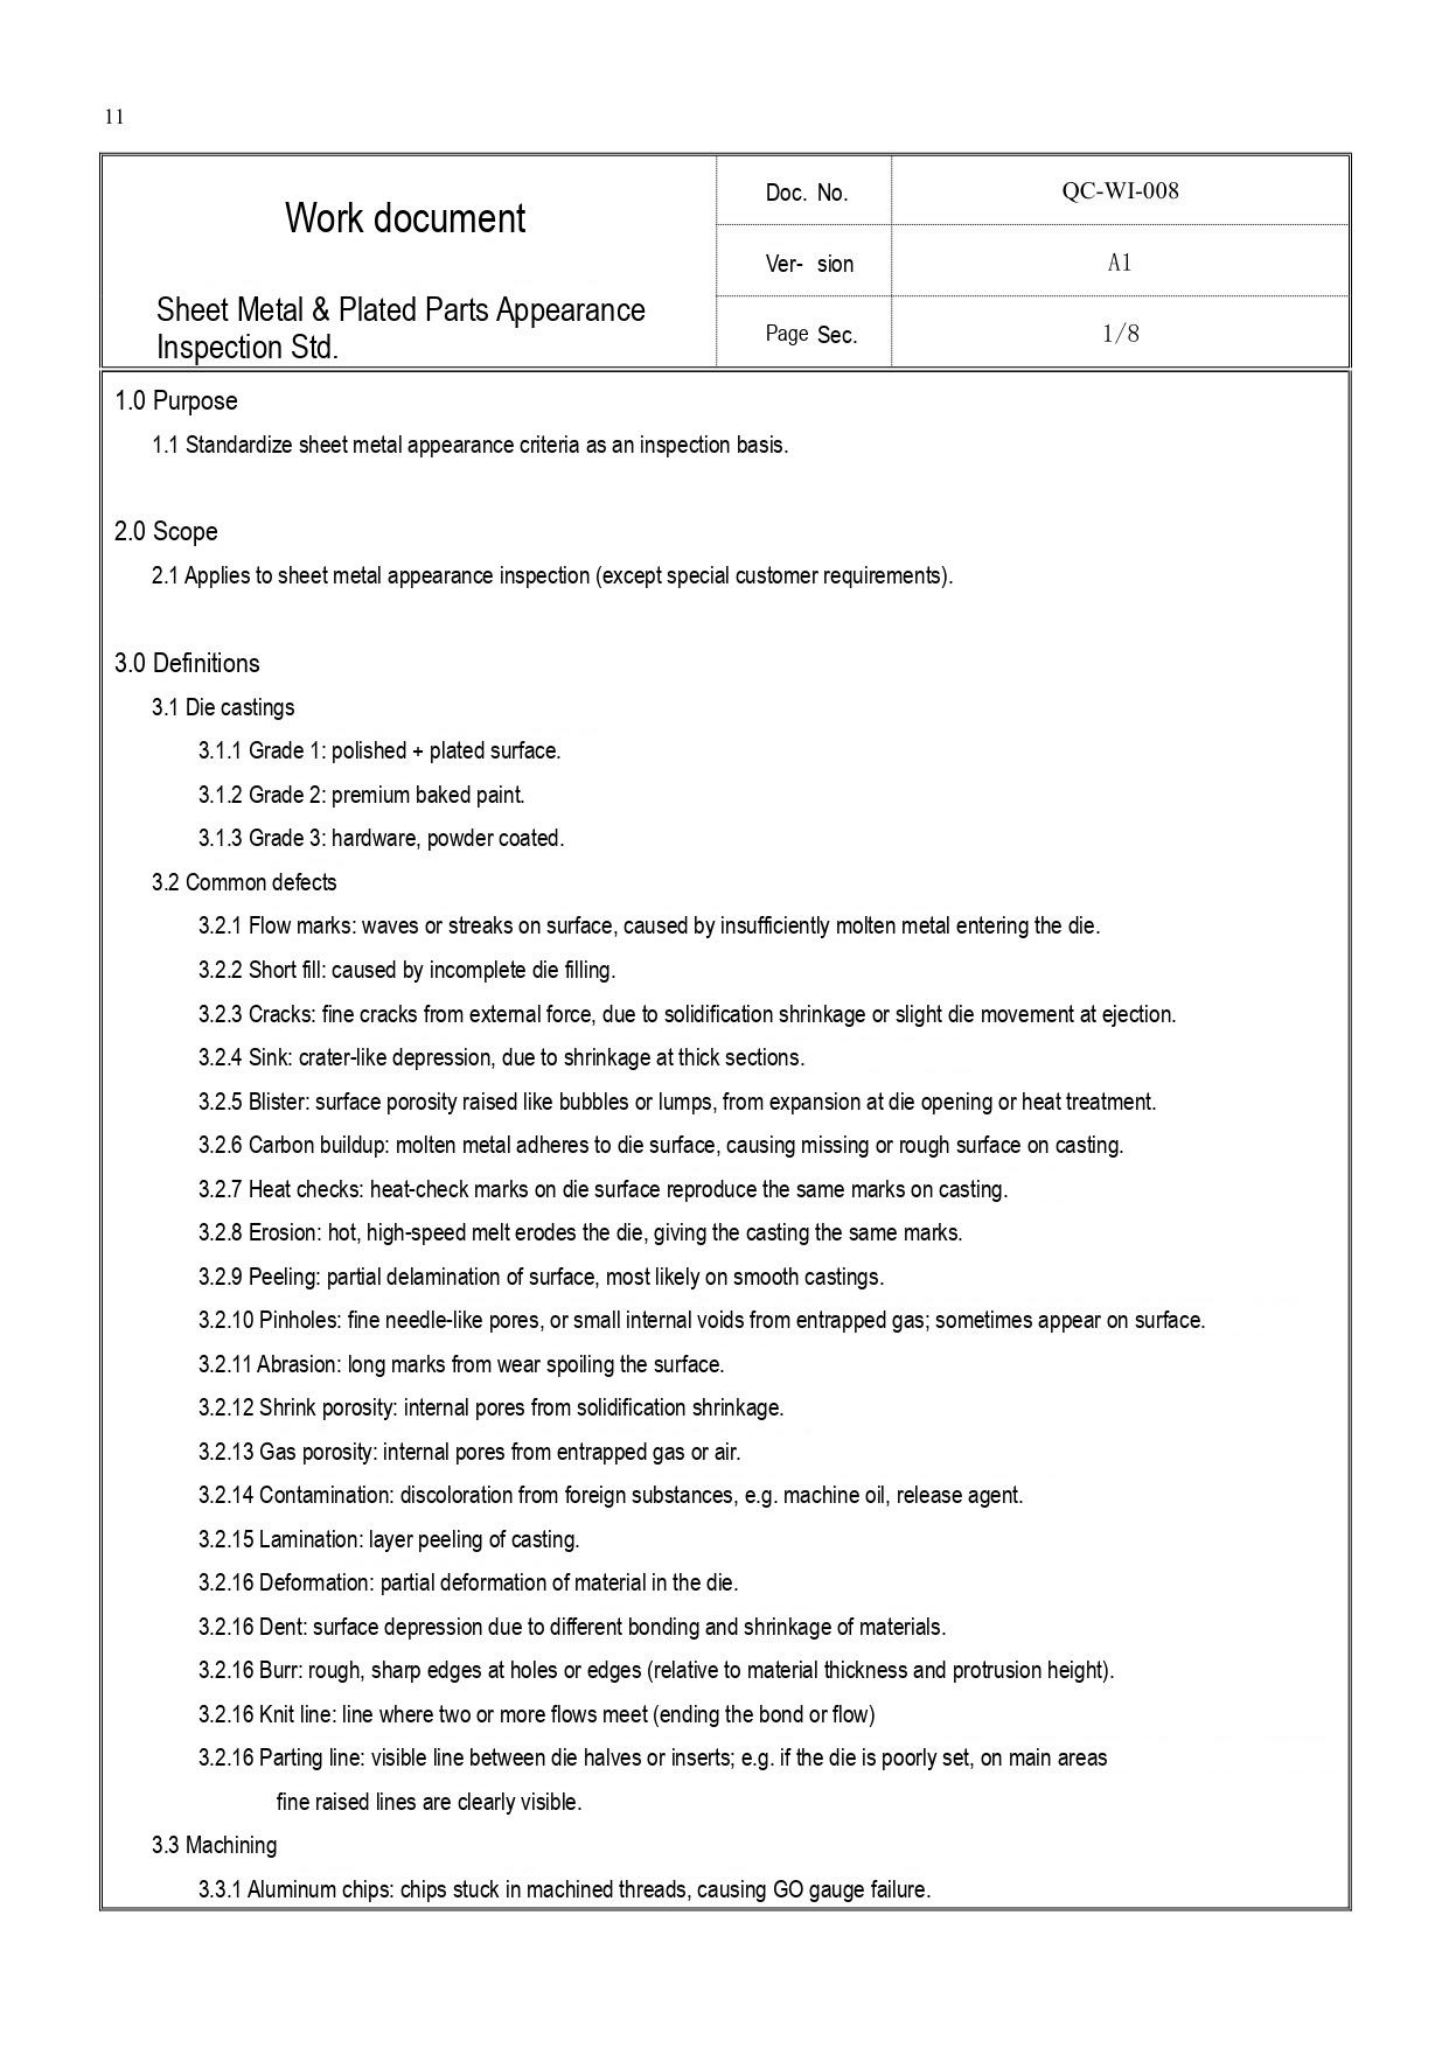11

| Work document<br><br>Sheet Metal & Plated Parts Appearance Inspection Std. | Doc. No. | QC-WI-008 |
|---|---|---|
| | Ver- sion | A1 |
| | Page Sec. | 1/8 |

1.0 Purpose

1.1 Standardize sheet metal appearance criteria as an inspection basis.

2.0 Scope

2.1 Applies to sheet metal appearance inspection (except special customer requirements).

3.0 Definitions

3.1 Die castings

3.1.1 Grade 1: polished + plated surface.

3.1.2 Grade 2: premium baked paint.

3.1.3 Grade 3: hardware, powder coated.

3.2 Common defects

3.2.1 Flow marks: waves or streaks on surface, caused by insufficiently molten metal entering the die.

3.2.2 Short fill: caused by incomplete die filling.

3.2.3 Cracks: fine cracks from external force, due to solidification shrinkage or slight die movement at ejection.

3.2.4 Sink: crater-like depression, due to shrinkage at thick sections.

3.2.5 Blister: surface porosity raised like bubbles or lumps, from expansion at die opening or heat treatment.

3.2.6 Carbon buildup: molten metal adheres to die surface, causing missing or rough surface on casting.

3.2.7 Heat checks: heat-check marks on die surface reproduce the same marks on casting.

3.2.8 Erosion: hot, high-speed melt erodes the die, giving the casting the same marks.

3.2.9 Peeling: partial delamination of surface, most likely on smooth castings.

3.2.10 Pinholes: fine needle-like pores, or small internal voids from entrapped gas; sometimes appear on surface.

3.2.11 Abrasion: long marks from wear spoiling the surface.

3.2.12 Shrink porosity: internal pores from solidification shrinkage.

3.2.13 Gas porosity: internal pores from entrapped gas or air.

3.2.14 Contamination: discoloration from foreign substances, e.g. machine oil, release agent.

3.2.15 Lamination: layer peeling of casting.

3.2.16 Deformation: partial deformation of material in the die.

3.2.16 Dent: surface depression due to different bonding and shrinkage of materials.

3.2.16 Burr: rough, sharp edges at holes or edges (relative to material thickness and protrusion height).

3.2.16 Knit line: line where two or more flows meet (ending the bond or flow)

3.2.16 Parting line: visible line between die halves or inserts; e.g. if the die is poorly set, on main areas fine raised lines are clearly visible.

3.3 Machining

3.3.1 Aluminum chips: chips stuck in machined threads, causing GO gauge failure.
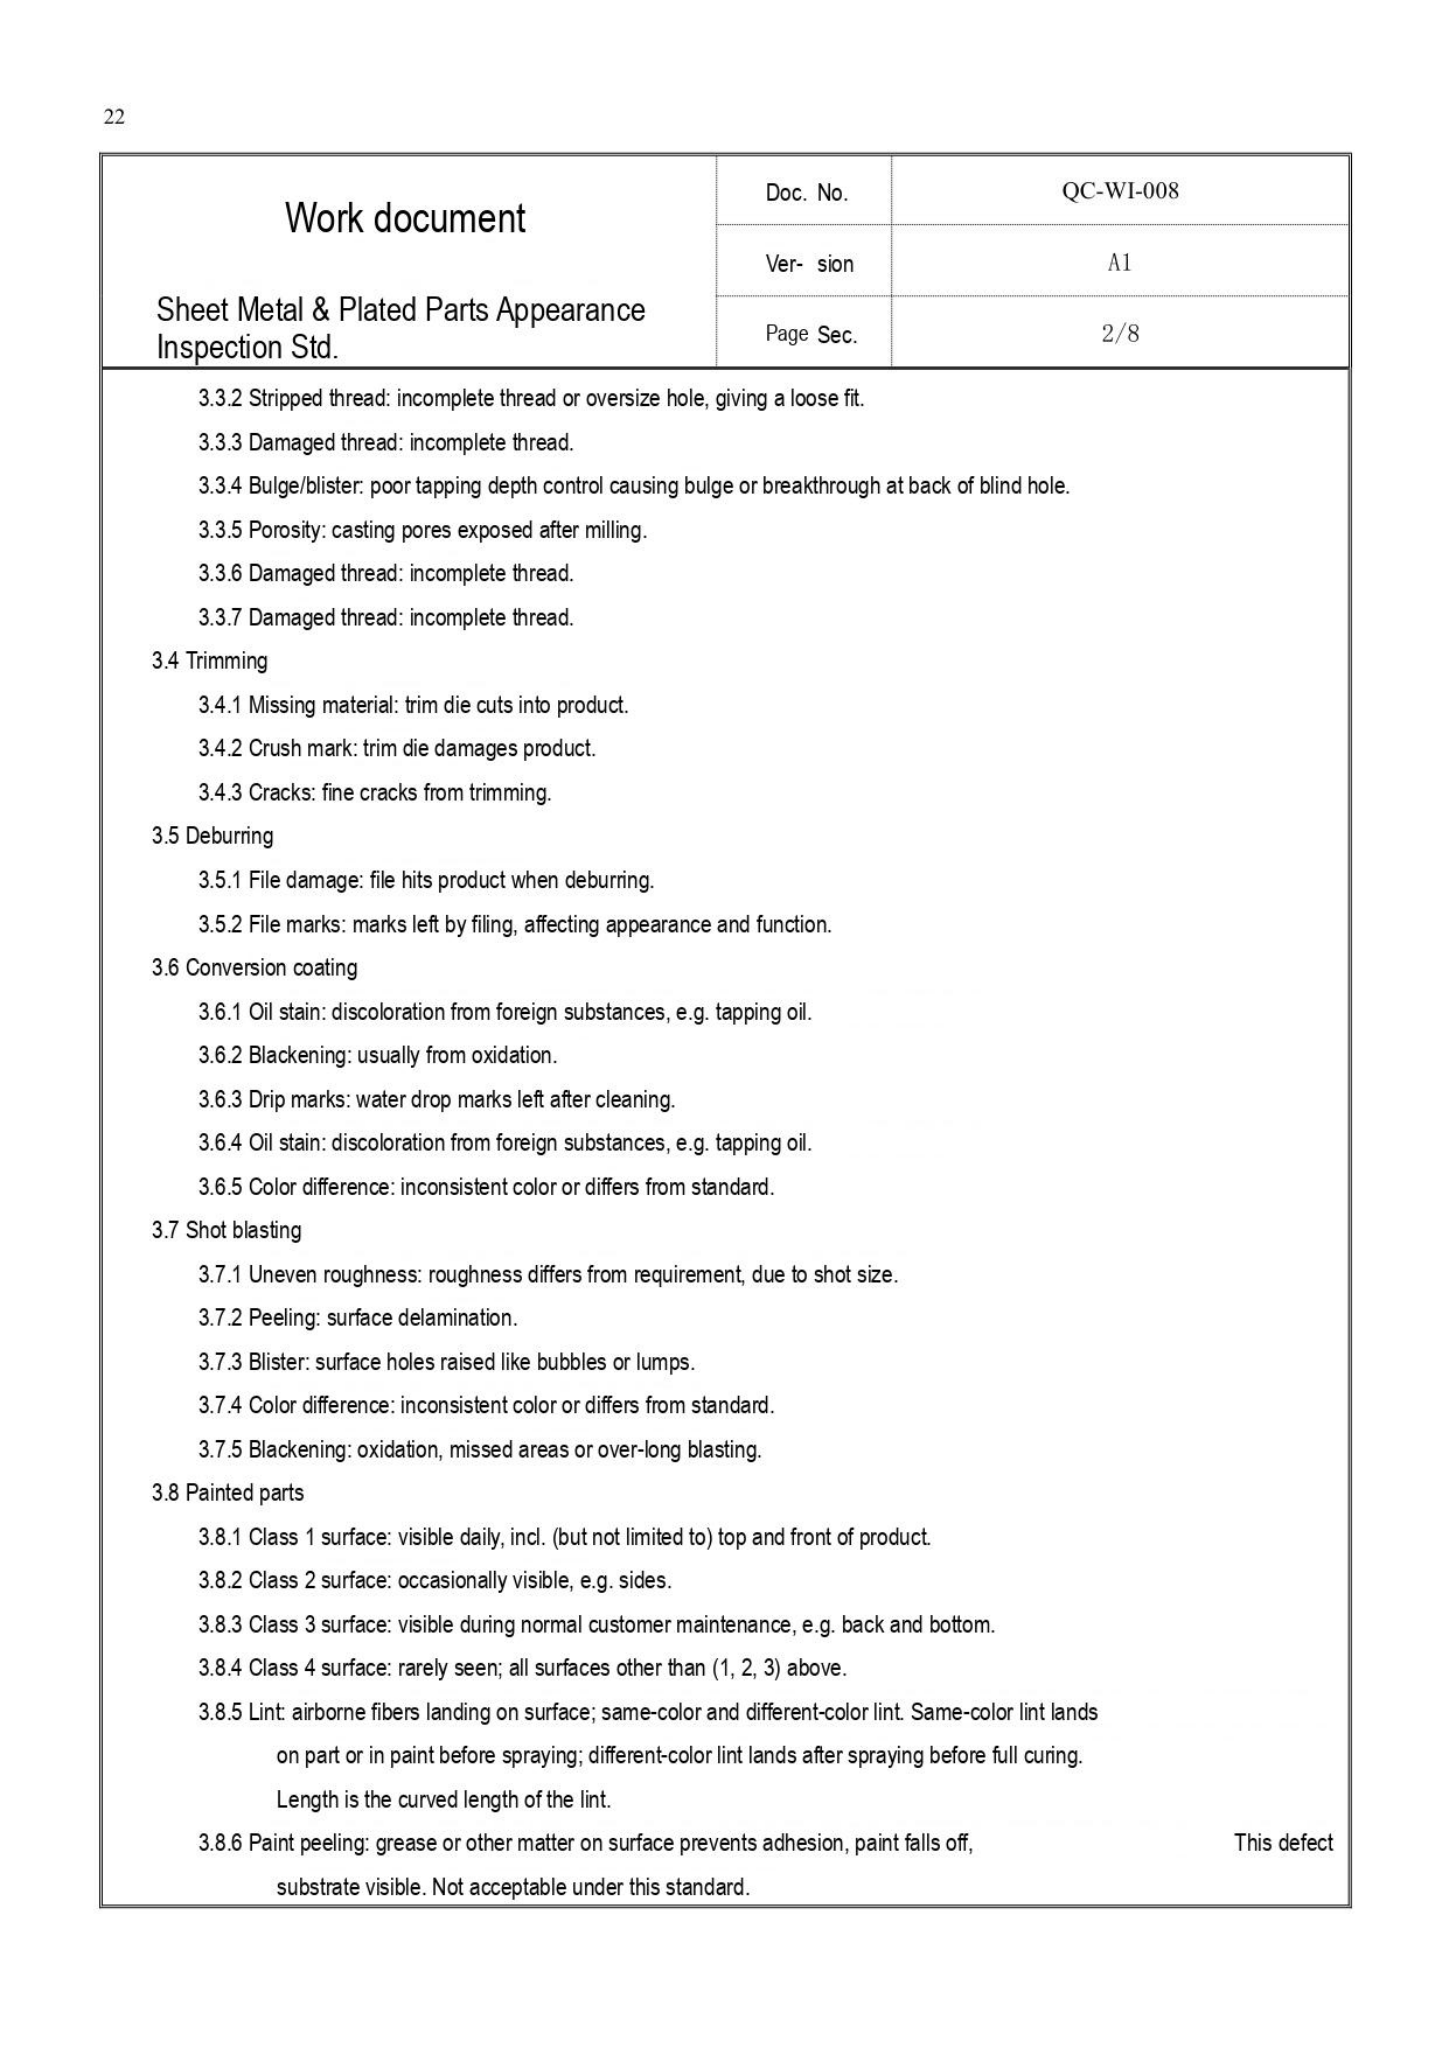22

| Work document<br><br>Sheet Metal & Plated Parts Appearance Inspection Std. | Doc. No. | QC-WI-008 |
|---|---|---|
| | Ver- sion | A1 |
| | Page Sec. | 2/8 |

3.3.2 Stripped thread: incomplete thread or oversize hole, giving a loose fit.

3.3.3 Damaged thread: incomplete thread.

3.3.4 Bulge/blister: poor tapping depth control causing bulge or breakthrough at back of blind hole.

3.3.5 Porosity: casting pores exposed after milling.

3.3.6 Damaged thread: incomplete thread.

3.3.7 Damaged thread: incomplete thread.

3.4 Trimming

3.4.1 Missing material: trim die cuts into product.

3.4.2 Crush mark: trim die damages product.

3.4.3 Cracks: fine cracks from trimming.

3.5 Deburring

3.5.1 File damage: file hits product when deburring.

3.5.2 File marks: marks left by filing, affecting appearance and function.

3.6 Conversion coating

3.6.1 Oil stain: discoloration from foreign substances, e.g. tapping oil.

3.6.2 Blackening: usually from oxidation.

3.6.3 Drip marks: water drop marks left after cleaning.

3.6.4 Oil stain: discoloration from foreign substances, e.g. tapping oil.

3.6.5 Color difference: inconsistent color or differs from standard.

3.7 Shot blasting

3.7.1 Uneven roughness: roughness differs from requirement, due to shot size.

3.7.2 Peeling: surface delamination.

3.7.3 Blister: surface holes raised like bubbles or lumps.

3.7.4 Color difference: inconsistent color or differs from standard.

3.7.5 Blackening: oxidation, missed areas or over-long blasting.

3.8 Painted parts

3.8.1 Class 1 surface: visible daily, incl. (but not limited to) top and front of product.

3.8.2 Class 2 surface: occasionally visible, e.g. sides.

3.8.3 Class 3 surface: visible during normal customer maintenance, e.g. back and bottom.

3.8.4 Class 4 surface: rarely seen; all surfaces other than (1, 2, 3) above.

3.8.5 Lint: airborne fibers landing on surface; same-color and different-color lint. Same-color lint lands on part or in paint before spraying; different-color lint lands after spraying before full curing. Length is the curved length of the lint.

3.8.6 Paint peeling: grease or other matter on surface prevents adhesion, paint falls off, substrate visible. Not acceptable under this standard.

This defect
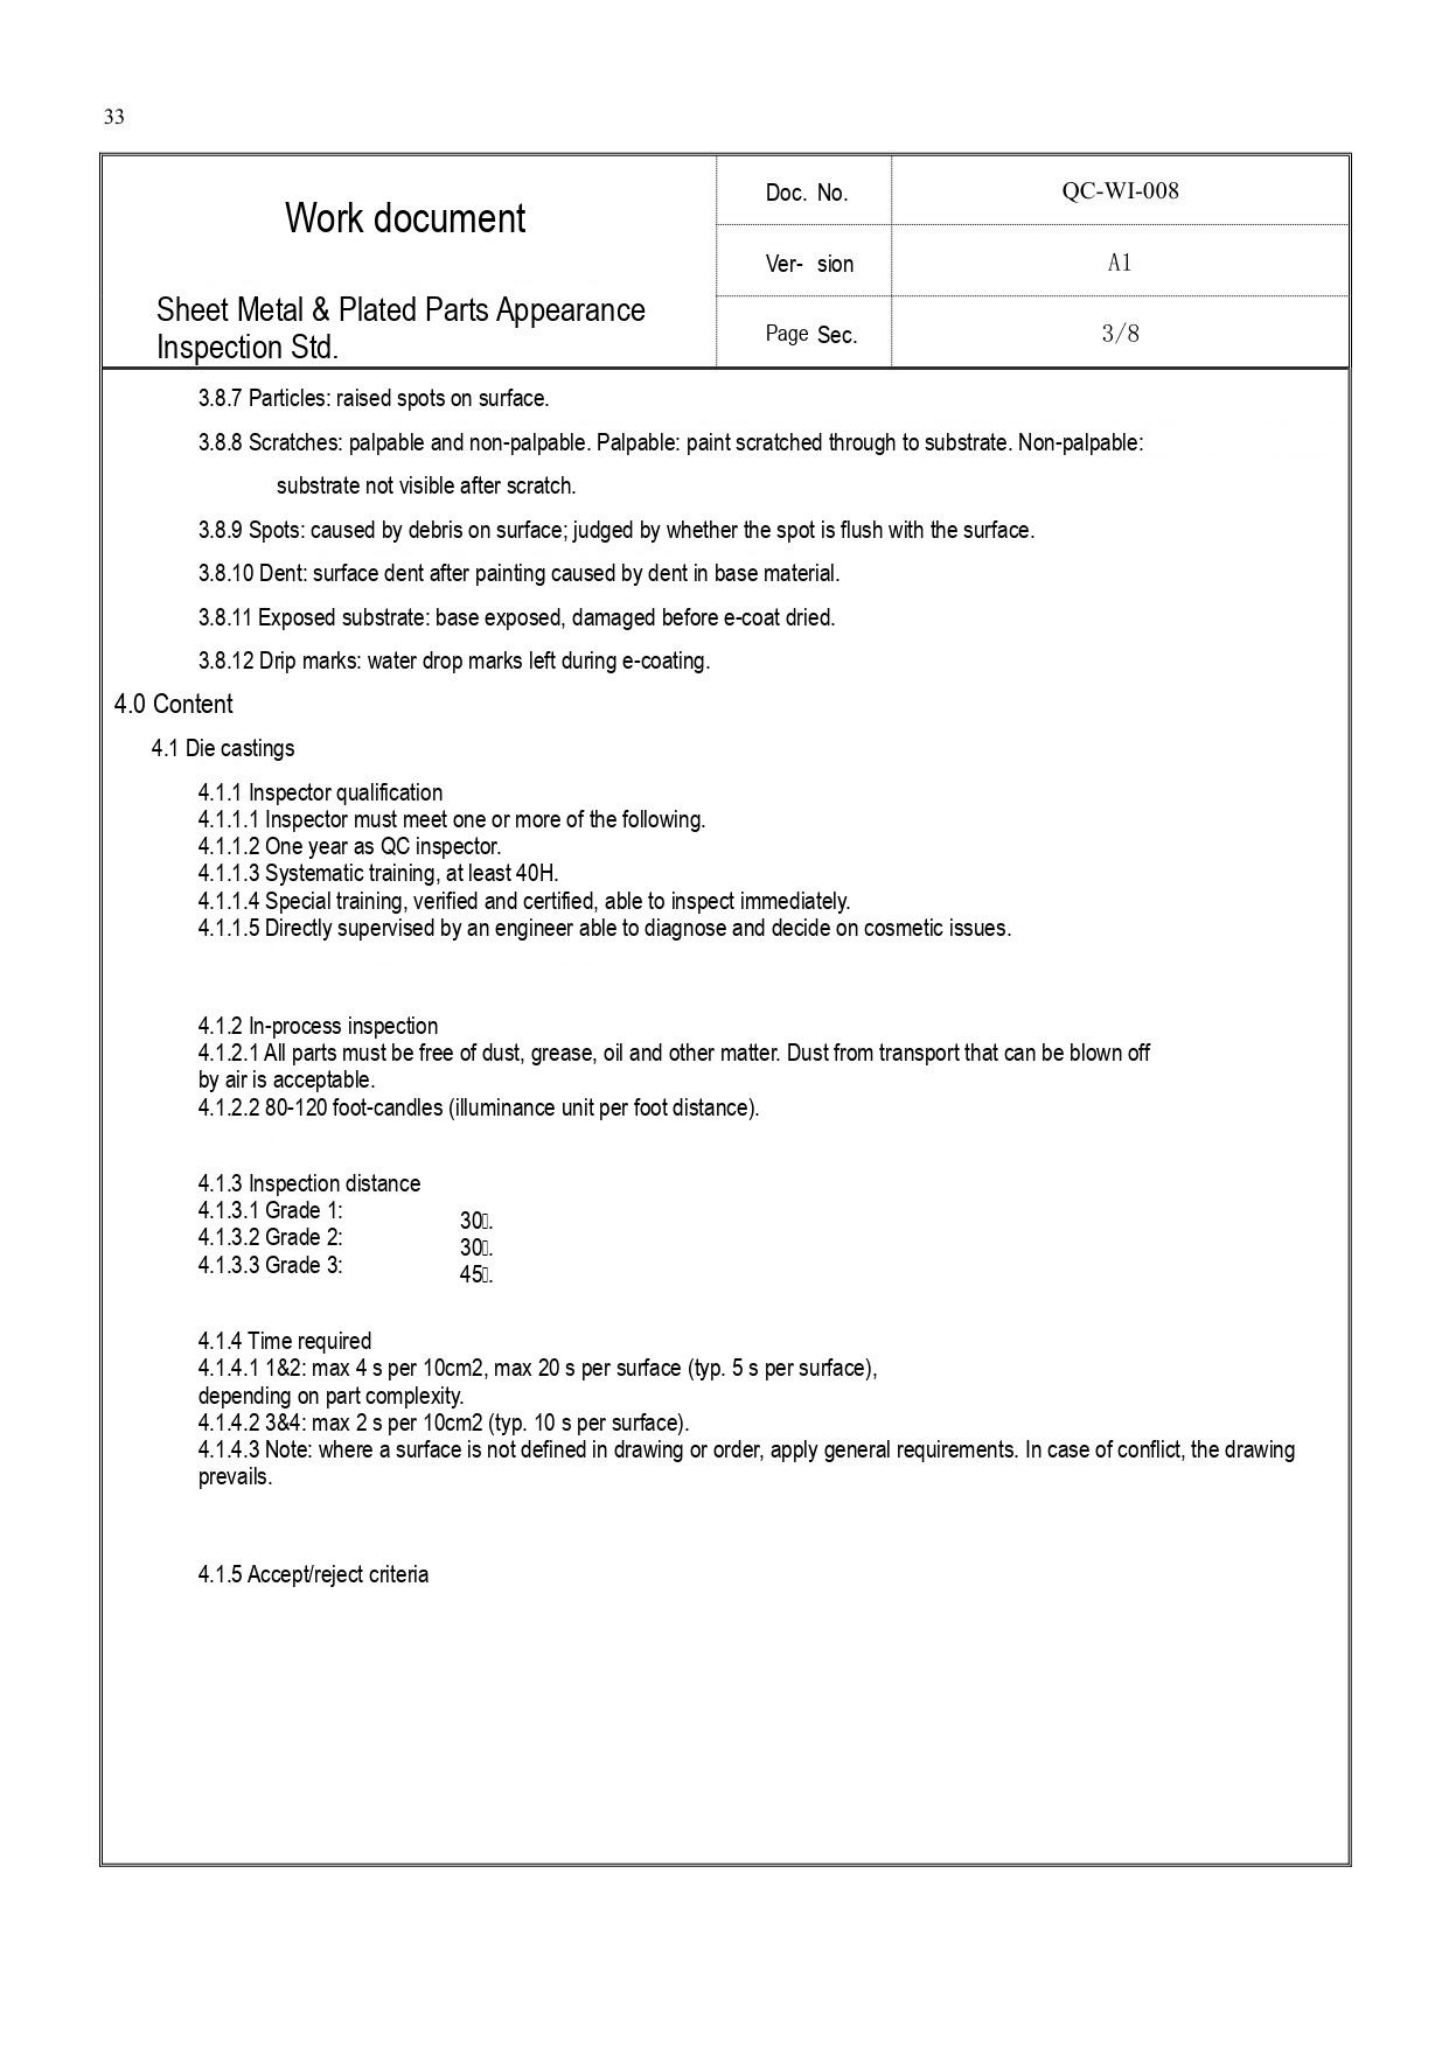33

| Work document<br><br>Sheet Metal & Plated Parts Appearance Inspection Std. | Doc. No. | QC-WI-008 |
|---|---|---|
| | Ver- sion | A1 |
| | Page Sec. | 3/8 |

3.8.7 Particles: raised spots on surface.

3.8.8 Scratches: palpable and non-palpable. Palpable: paint scratched through to substrate. Non-palpable: substrate not visible after scratch.

3.8.9 Spots: caused by debris on surface; judged by whether the spot is flush with the surface.

3.8.10 Dent: surface dent after painting caused by dent in base material.

3.8.11 Exposed substrate: base exposed, damaged before e-coat dried.

3.8.12 Drip marks: water drop marks left during e-coating.

4.0 Content

4.1 Die castings

4.1.1 Inspector qualification
4.1.1.1 Inspector must meet one or more of the following.
4.1.1.2 One year as QC inspector.
4.1.1.3 Systematic training, at least 40H.
4.1.1.4 Special training, verified and certified, able to inspect immediately.
4.1.1.5 Directly supervised by an engineer able to diagnose and decide on cosmetic issues.

4.1.2 In-process inspection
4.1.2.1 All parts must be free of dust, grease, oil and other matter. Dust from transport that can be blown off by air is acceptable.
4.1.2.2 80-120 foot-candles (illuminance unit per foot distance).

4.1.3 Inspection distance
4.1.3.1 Grade 1: 30.
4.1.3.2 Grade 2: 30.
4.1.3.3 Grade 3: 45.

4.1.4 Time required
4.1.4.1 1&2: max 4 s per 10cm2, max 20 s per surface (typ. 5 s per surface), depending on part complexity.
4.1.4.2 3&4: max 2 s per 10cm2 (typ. 10 s per surface).
4.1.4.3 Note: where a surface is not defined in drawing or order, apply general requirements. In case of conflict, the drawing prevails.

4.1.5 Accept/reject criteria
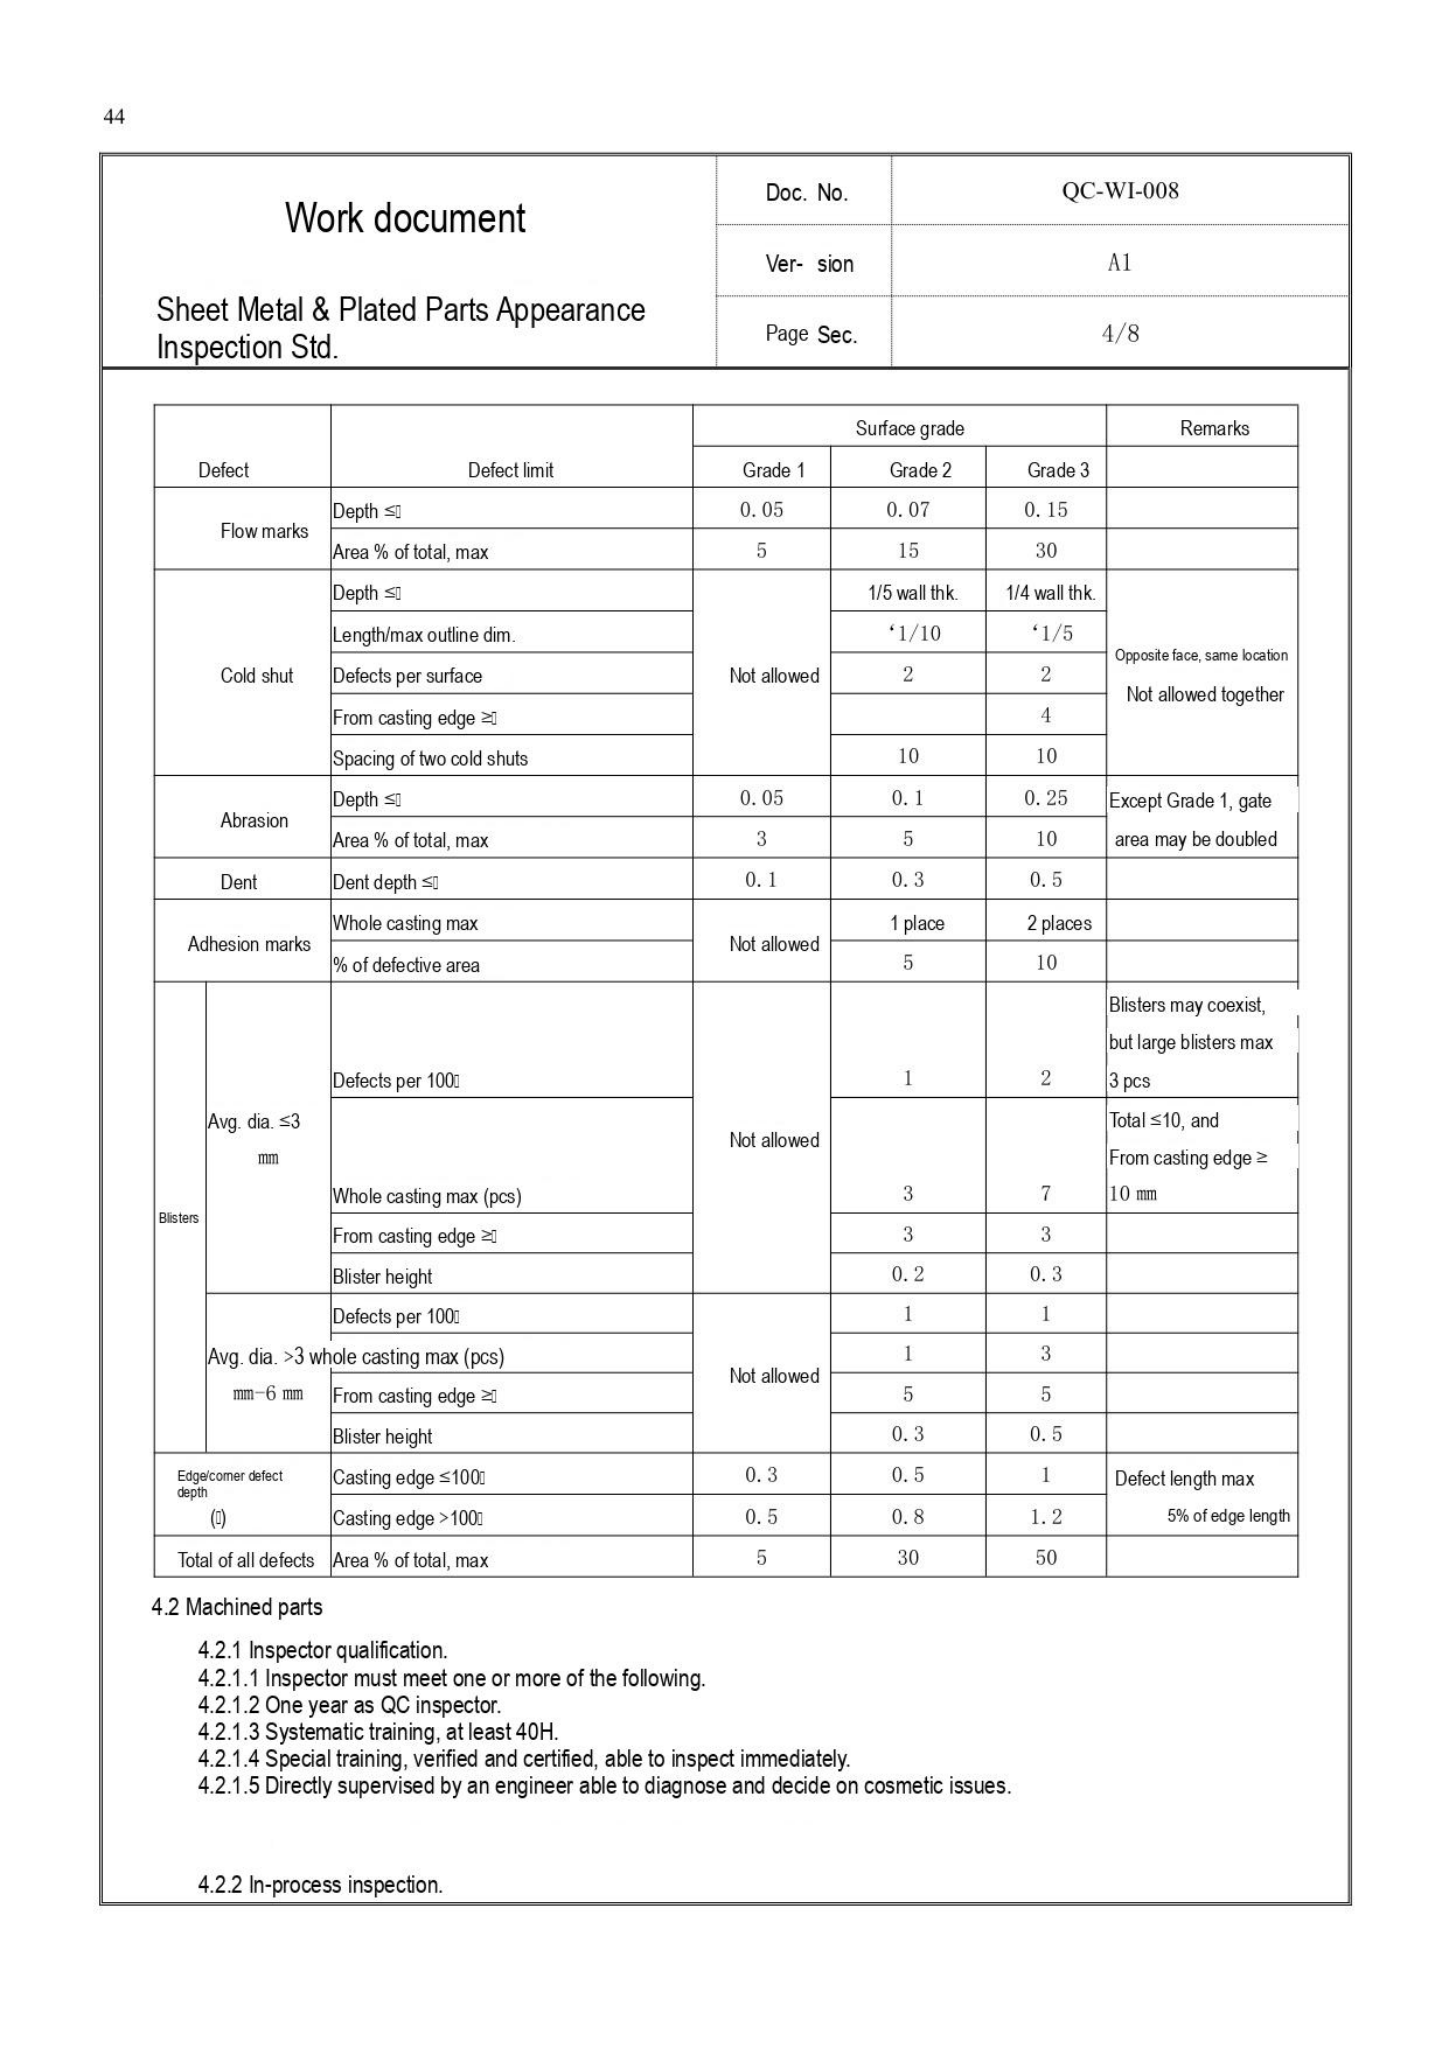44

| Work document | Doc. No. | QC-WI-008 |
|---|---|---|
| | Ver- sion | A1 |
| Sheet Metal & Plated Parts Appearance Inspection Std. | Page Sec. | 4/8 |

| Defect | | Defect limit | Surface grade: Grade 1 | Surface grade: Grade 2 | Surface grade: Grade 3 | Remarks |
|---|---|---|---|---|---|---|
| Flow marks | | Depth ≤ | 0. 05 | 0. 07 | 0. 15 | |
| Flow marks | | Area % of total, max | 5 | 15 | 30 | |
| Cold shut | | Depth ≤ | Not allowed | 1/5 wall thk. | 1/4 wall thk. | Opposite face, same location Not allowed together |
| Cold shut | | Length/max outline dim. | Not allowed | ‘1/10 | ‘1/5 | Opposite face, same location Not allowed together |
| Cold shut | | Defects per surface | Not allowed | 2 | 2 | Opposite face, same location Not allowed together |
| Cold shut | | From casting edge ≥ | Not allowed | | 4 | Opposite face, same location Not allowed together |
| Cold shut | | Spacing of two cold shuts | Not allowed | 10 | 10 | Opposite face, same location Not allowed together |
| Abrasion | | Depth ≤ | 0. 05 | 0. 1 | 0. 25 | Except Grade 1, gate area may be doubled |
| Abrasion | | Area % of total, max | 3 | 5 | 10 | Except Grade 1, gate area may be doubled |
| Dent | | Dent depth ≤ | 0. 1 | 0. 3 | 0. 5 | |
| Adhesion marks | | Whole casting max | Not allowed | 1 place | 2 places | |
| Adhesion marks | | % of defective area | Not allowed | 5 | 10 | |
| Blisters | Avg. dia. ≤3 mm | Defects per 100 | Not allowed | 1 | 2 | Blisters may coexist, but large blisters max 3 pcs |
| Blisters | Avg. dia. ≤3 mm | Whole casting max (pcs) | Not allowed | 3 | 7 | Total ≤10, and From casting edge ≥ 10 mm |
| Blisters | Avg. dia. ≤3 mm | From casting edge ≥ | Not allowed | 3 | 3 | |
| Blisters | Avg. dia. ≤3 mm | Blister height | Not allowed | 0. 2 | 0. 3 | |
| Blisters | Avg. dia. >3 mm–6 mm | Defects per 100 | Not allowed | 1 | 1 | |
| Blisters | Avg. dia. >3 mm–6 mm | whole casting max (pcs) | Not allowed | 1 | 3 | |
| Blisters | Avg. dia. >3 mm–6 mm | From casting edge ≥ | Not allowed | 5 | 5 | |
| Blisters | Avg. dia. >3 mm–6 mm | Blister height | Not allowed | 0. 3 | 0. 5 | |
| Edge/corner defect depth () | | Casting edge ≤100 | 0. 3 | 0. 5 | 1 | Defect length max 5% of edge length |
| Edge/corner defect depth () | | Casting edge >100 | 0. 5 | 0. 8 | 1. 2 | Defect length max 5% of edge length |
| Total of all defects | | Area % of total, max | 5 | 30 | 50 | |

4.2 Machined parts

4.2.1 Inspector qualification.
4.2.1.1 Inspector must meet one or more of the following.
4.2.1.2 One year as QC inspector.
4.2.1.3 Systematic training, at least 40H.
4.2.1.4 Special training, verified and certified, able to inspect immediately.
4.2.1.5 Directly supervised by an engineer able to diagnose and decide on cosmetic issues.

4.2.2 In-process inspection.
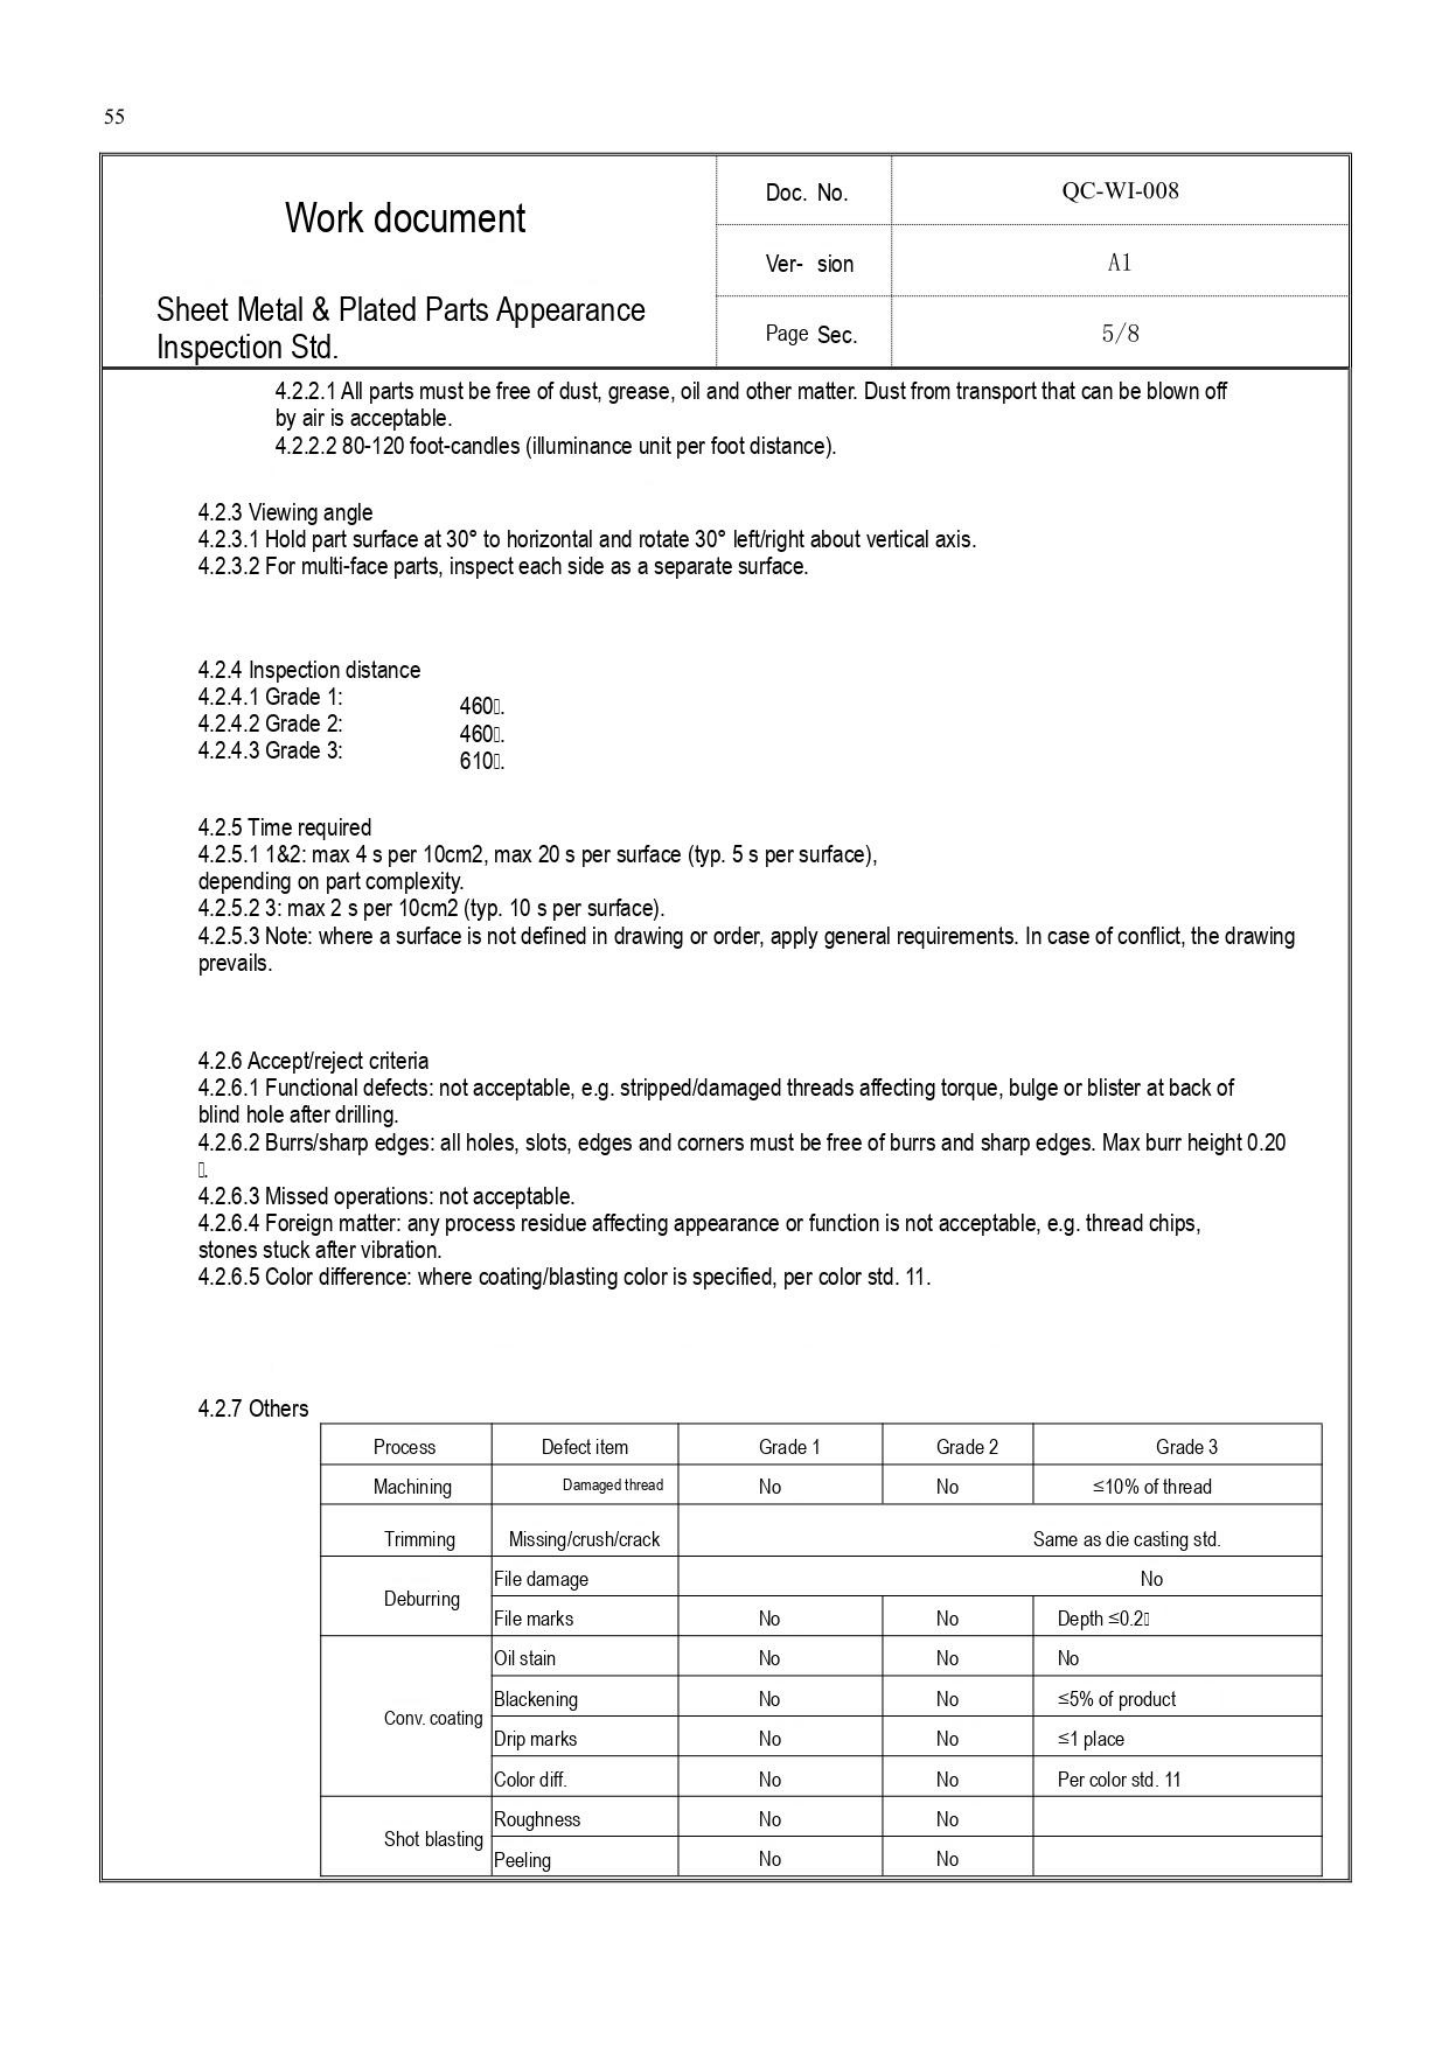55

| Work document | Doc. No. | QC-WI-008 |
|---|---|---|
| | Ver- sion | A1 |
| Sheet Metal & Plated Parts Appearance Inspection Std. | Page Sec. | 5/8 |

4.2.2.1 All parts must be free of dust, grease, oil and other matter. Dust from transport that can be blown off by air is acceptable.
4.2.2.2 80-120 foot-candles (illuminance unit per foot distance).

4.2.3 Viewing angle
4.2.3.1 Hold part surface at 30° to horizontal and rotate 30° left/right about vertical axis.
4.2.3.2 For multi-face parts, inspect each side as a separate surface.

4.2.4 Inspection distance
4.2.4.1 Grade 1: 460.
4.2.4.2 Grade 2: 460.
4.2.4.3 Grade 3: 610.

4.2.5 Time required
4.2.5.1 1&2: max 4 s per 10cm2, max 20 s per surface (typ. 5 s per surface), depending on part complexity.
4.2.5.2 3: max 2 s per 10cm2 (typ. 10 s per surface).
4.2.5.3 Note: where a surface is not defined in drawing or order, apply general requirements. In case of conflict, the drawing prevails.

4.2.6 Accept/reject criteria
4.2.6.1 Functional defects: not acceptable, e.g. stripped/damaged threads affecting torque, bulge or blister at back of blind hole after drilling.
4.2.6.2 Burrs/sharp edges: all holes, slots, edges and corners must be free of burrs and sharp edges. Max burr height 0.20
4.2.6.3 Missed operations: not acceptable.
4.2.6.4 Foreign matter: any process residue affecting appearance or function is not acceptable, e.g. thread chips, stones stuck after vibration.
4.2.6.5 Color difference: where coating/blasting color is specified, per color std. 11.

4.2.7 Others

| Process | Defect item | Grade 1 | Grade 2 | Grade 3 |
|---|---|---|---|---|
| Machining | Damaged thread | No | No | ≤10% of thread |
| Trimming | Missing/crush/crack | Same as die casting std. | | |
| Deburring | File damage | No | | |
| | File marks | No | No | Depth ≤0.2 |
| Conv. coating | Oil stain | No | No | No |
| | Blackening | No | No | ≤5% of product |
| | Drip marks | No | No | ≤1 place |
| | Color diff. | No | No | Per color std. 11 |
| Shot blasting | Roughness | No | No | |
| | Peeling | No | No | |
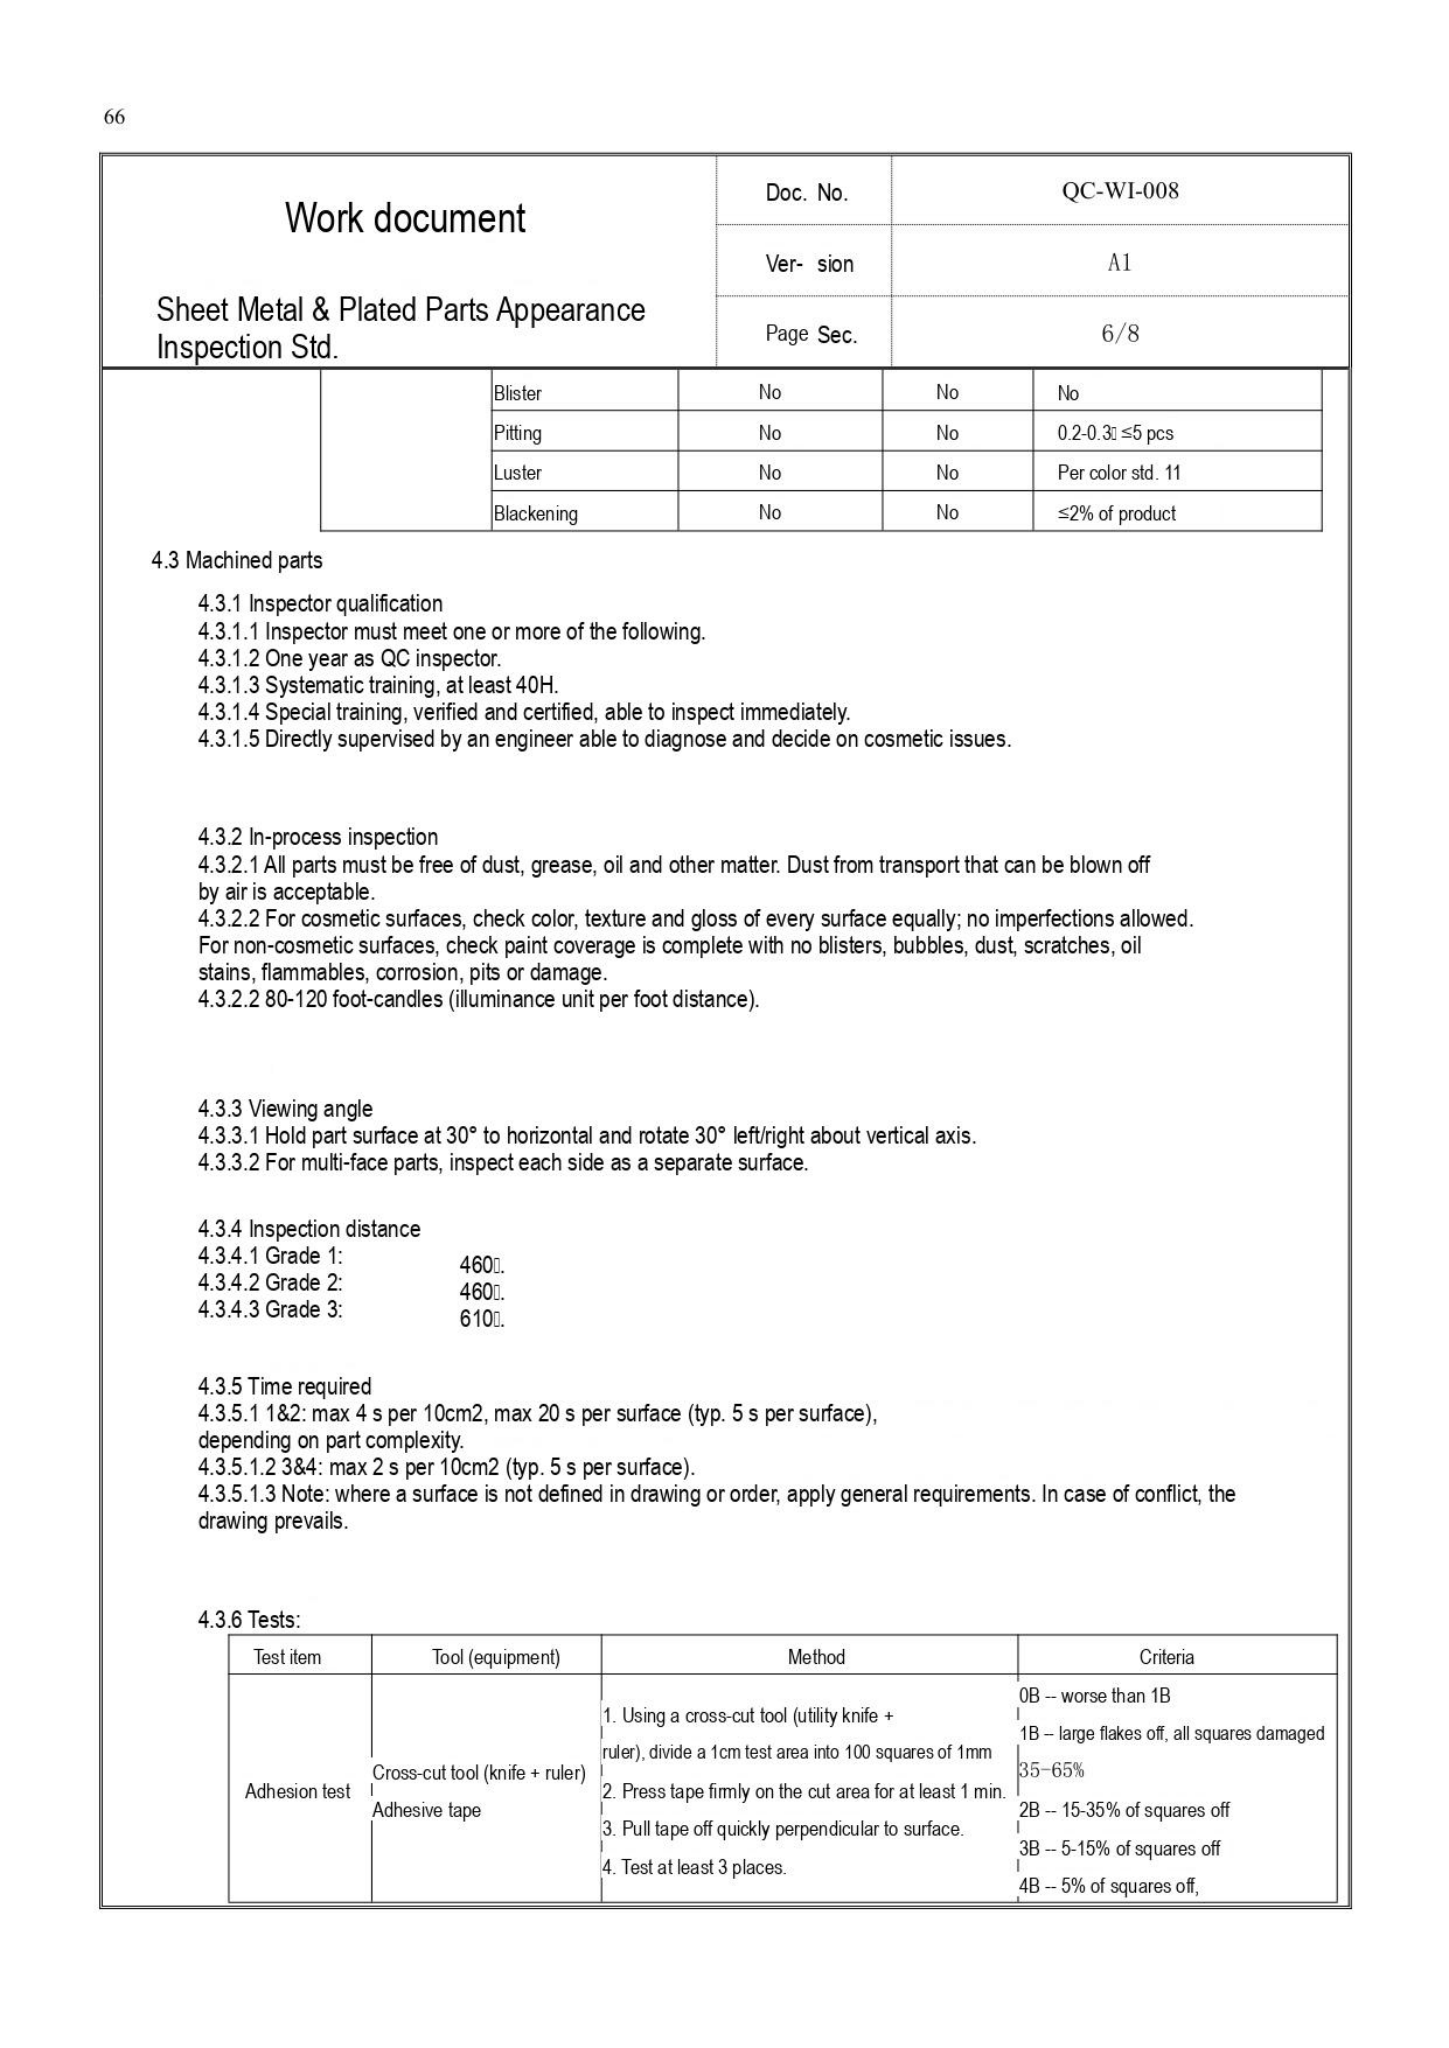66

| Work document<br><br>Sheet Metal & Plated Parts Appearance Inspection Std. | Doc. No. | QC-WI-008 |
|---|---|---|
| | Ver- sion | A1 |
| | Page Sec. | 6/8 |

| | | | | |
|---|---|---|---|---|
| | Blister | No | No | No |
| | Pitting | No | No | 0.2-0.3 ≤5 pcs |
| | Luster | No | No | Per color std. 11 |
| | Blackening | No | No | ≤2% of product |

4.3 Machined parts

4.3.1 Inspector qualification
4.3.1.1 Inspector must meet one or more of the following.
4.3.1.2 One year as QC inspector.
4.3.1.3 Systematic training, at least 40H.
4.3.1.4 Special training, verified and certified, able to inspect immediately.
4.3.1.5 Directly supervised by an engineer able to diagnose and decide on cosmetic issues.

4.3.2 In-process inspection
4.3.2.1 All parts must be free of dust, grease, oil and other matter. Dust from transport that can be blown off by air is acceptable.
4.3.2.2 For cosmetic surfaces, check color, texture and gloss of every surface equally; no imperfections allowed. For non-cosmetic surfaces, check paint coverage is complete with no blisters, bubbles, dust, scratches, oil stains, flammables, corrosion, pits or damage.
4.3.2.2 80-120 foot-candles (illuminance unit per foot distance).

4.3.3 Viewing angle
4.3.3.1 Hold part surface at 30° to horizontal and rotate 30° left/right about vertical axis.
4.3.3.2 For multi-face parts, inspect each side as a separate surface.

4.3.4 Inspection distance
4.3.4.1 Grade 1: 460.
4.3.4.2 Grade 2: 460.
4.3.4.3 Grade 3: 610.

4.3.5 Time required
4.3.5.1 1&2: max 4 s per 10cm2, max 20 s per surface (typ. 5 s per surface), depending on part complexity.
4.3.5.1.2 3&4: max 2 s per 10cm2 (typ. 5 s per surface).
4.3.5.1.3 Note: where a surface is not defined in drawing or order, apply general requirements. In case of conflict, the drawing prevails.

4.3.6 Tests:

| Test item | Tool (equipment) | Method | Criteria |
|---|---|---|---|
| Adhesion test | Cross-cut tool (knife + ruler)<br>Adhesive tape | 1. Using a cross-cut tool (utility knife + ruler), divide a 1cm test area into 100 squares of 1mm<br>2. Press tape firmly on the cut area for at least 1 min.<br>3. Pull tape off quickly perpendicular to surface.<br>4. Test at least 3 places. | 0B -- worse than 1B<br>1B – large flakes off, all squares damaged 35-65%<br>2B -- 15-35% of squares off<br>3B -- 5-15% of squares off<br>4B -- 5% of squares off, |